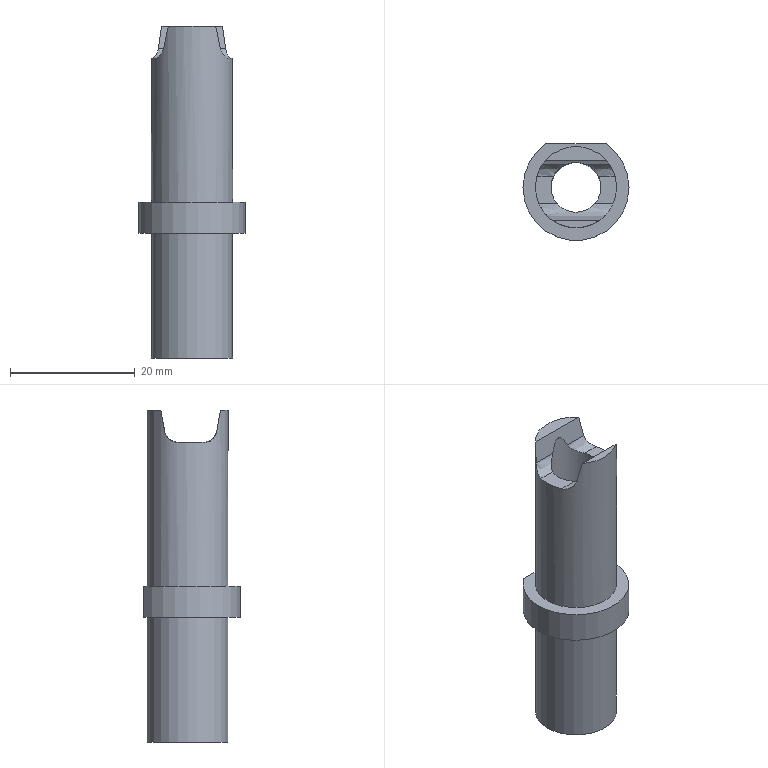Part | STEP file | P011002M013-000 | 1 solid | 17 faces | box 17 x 15.5 x 53.228 mm | volume 4545 mm3 | plane 8 | spline 5 | cylinder 4 | commonest cylinder face diameters 13 x2 8 x1 17 x1